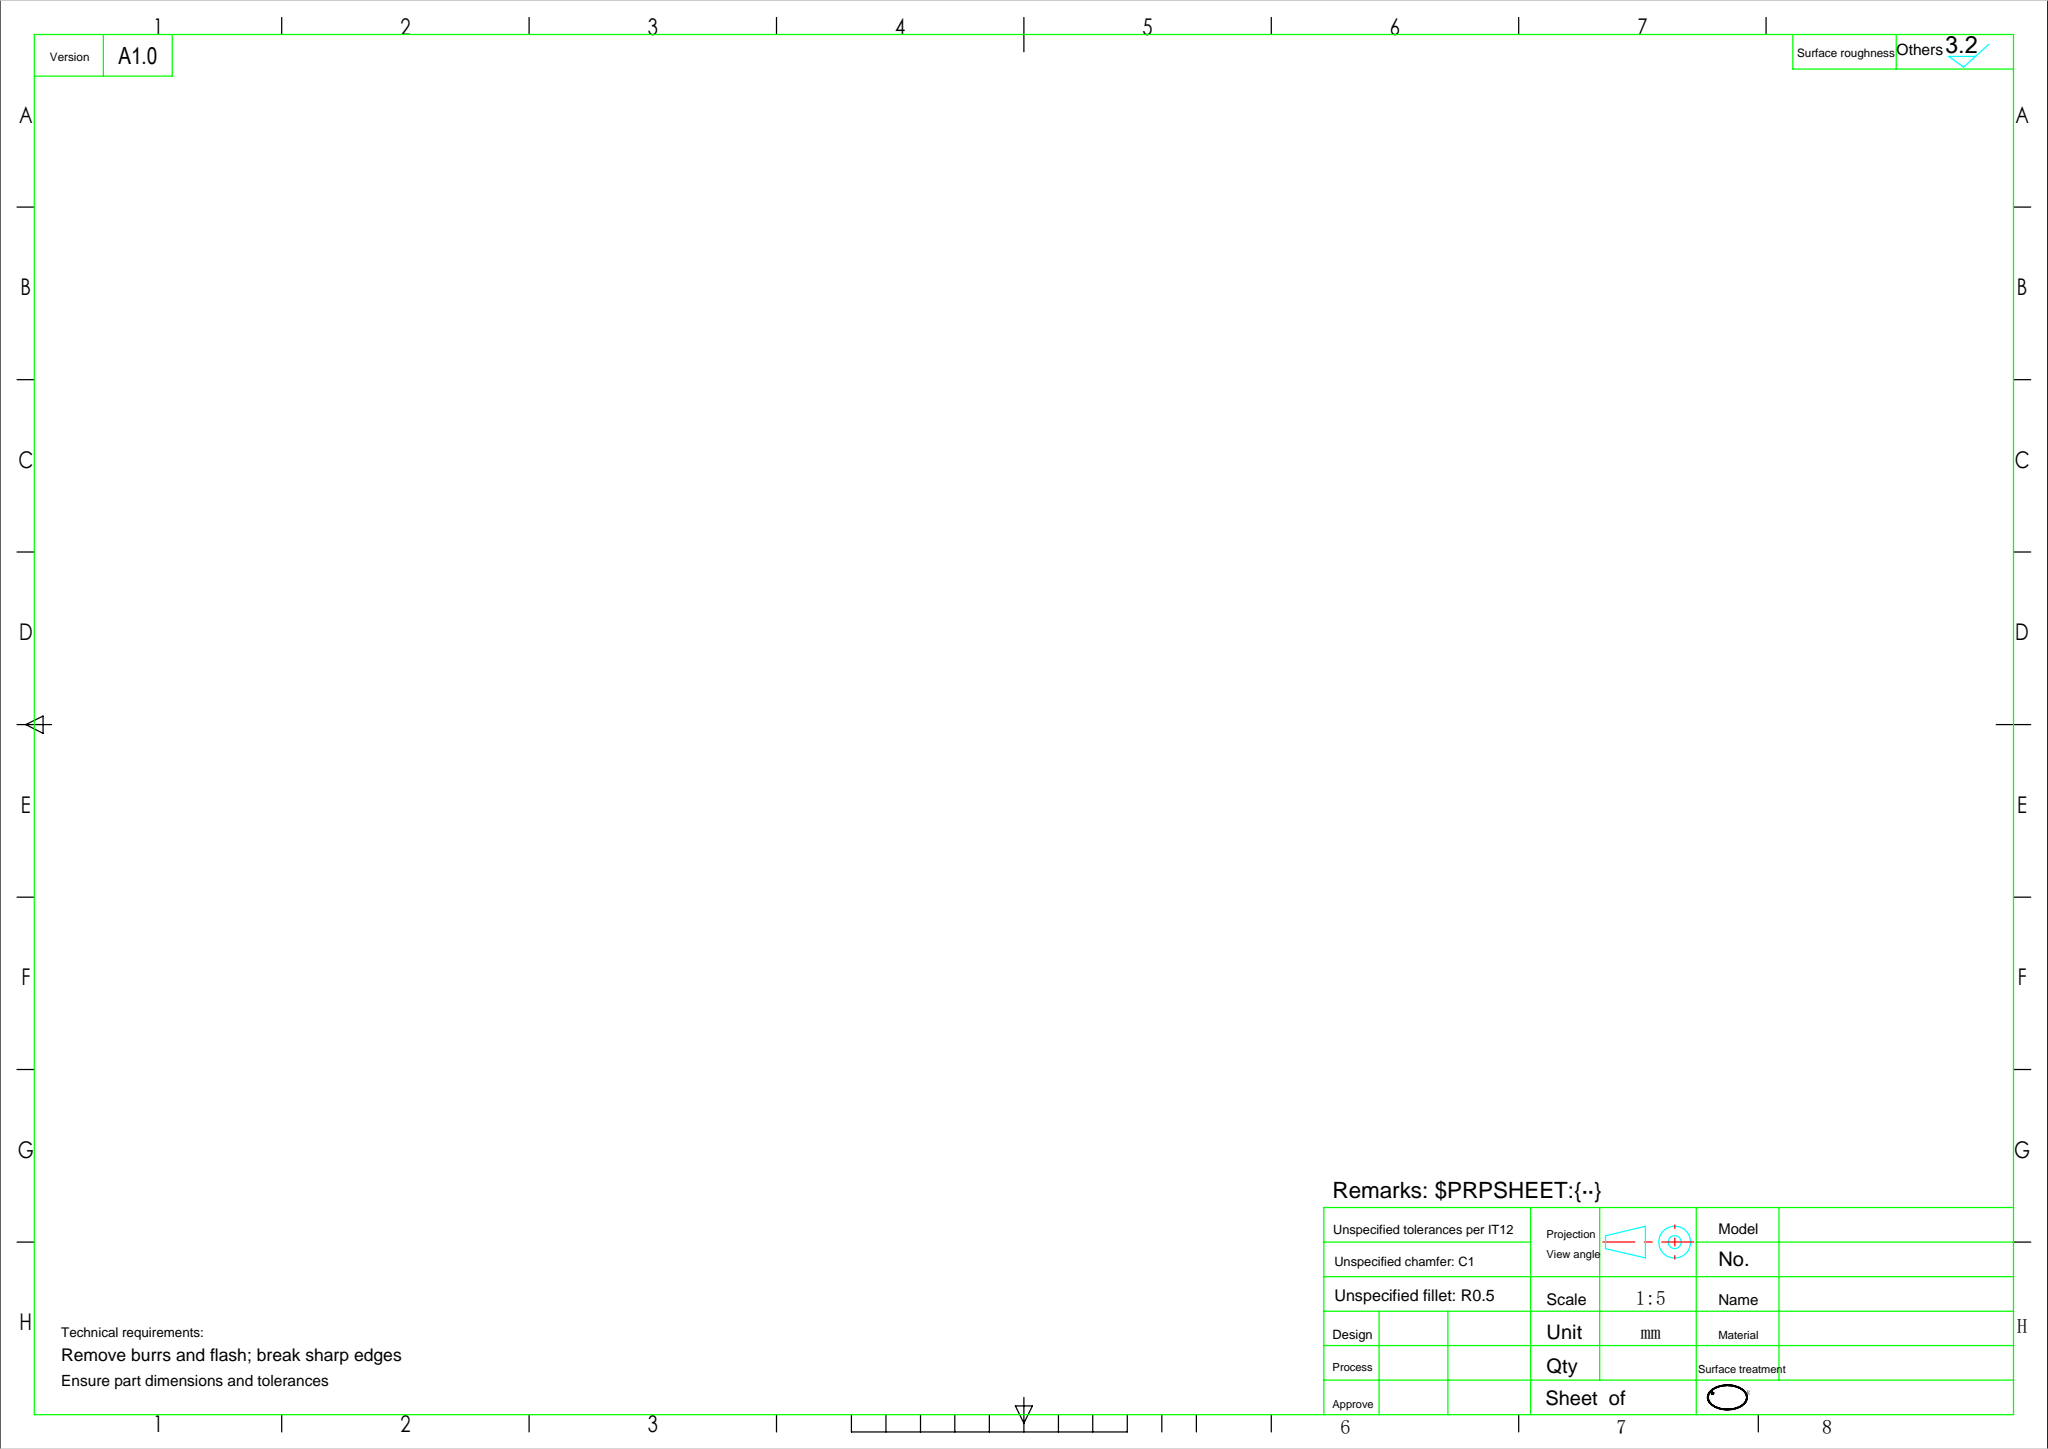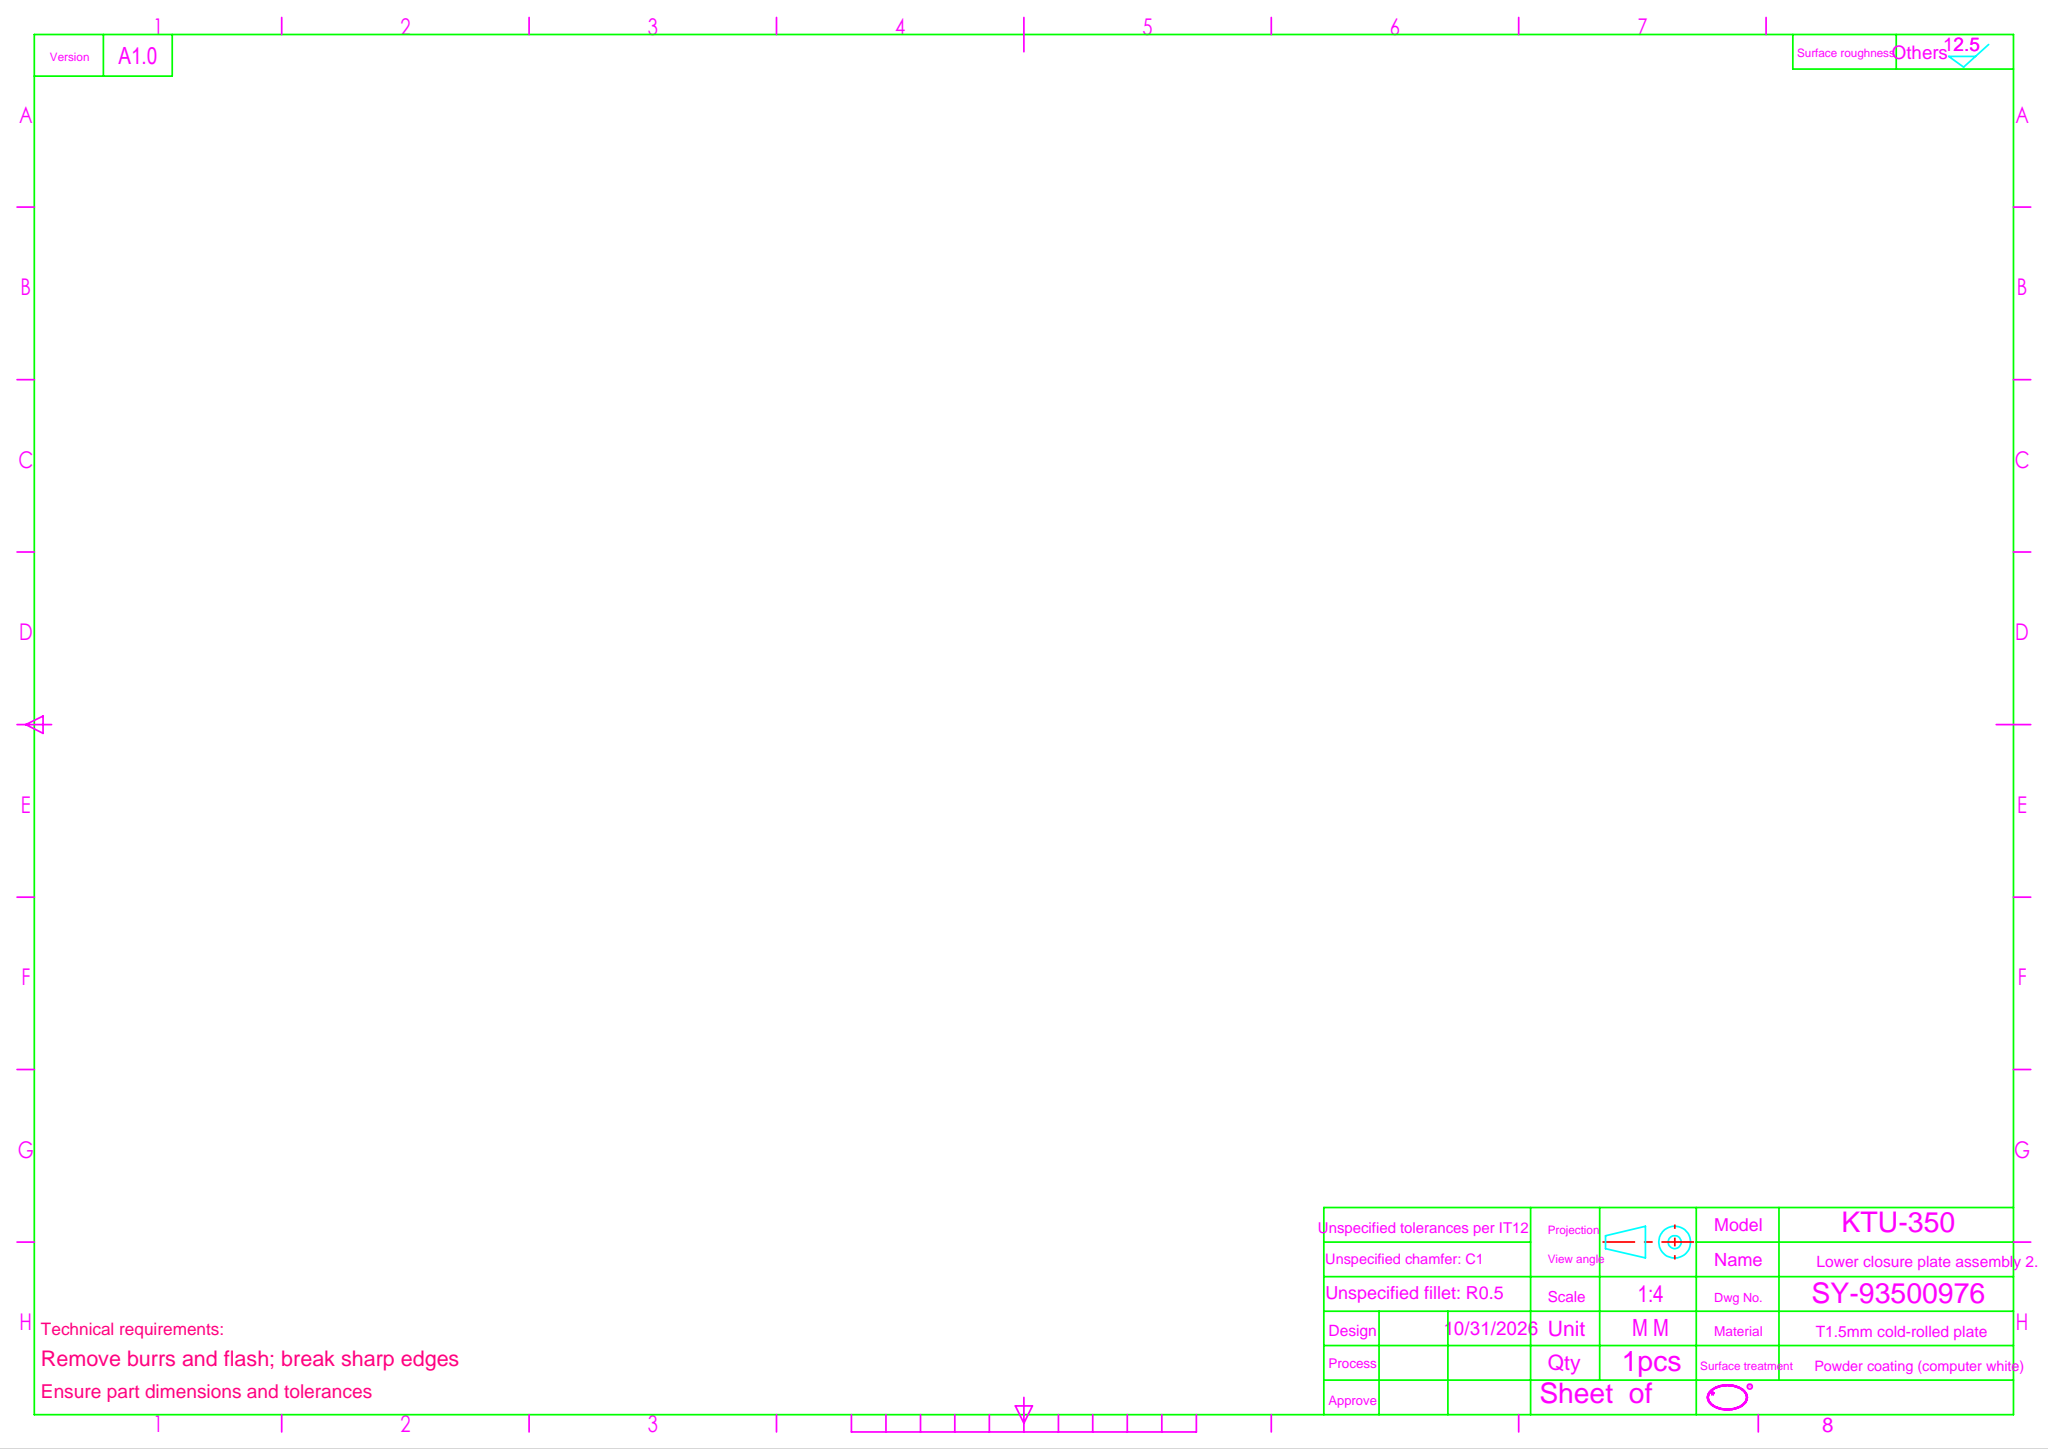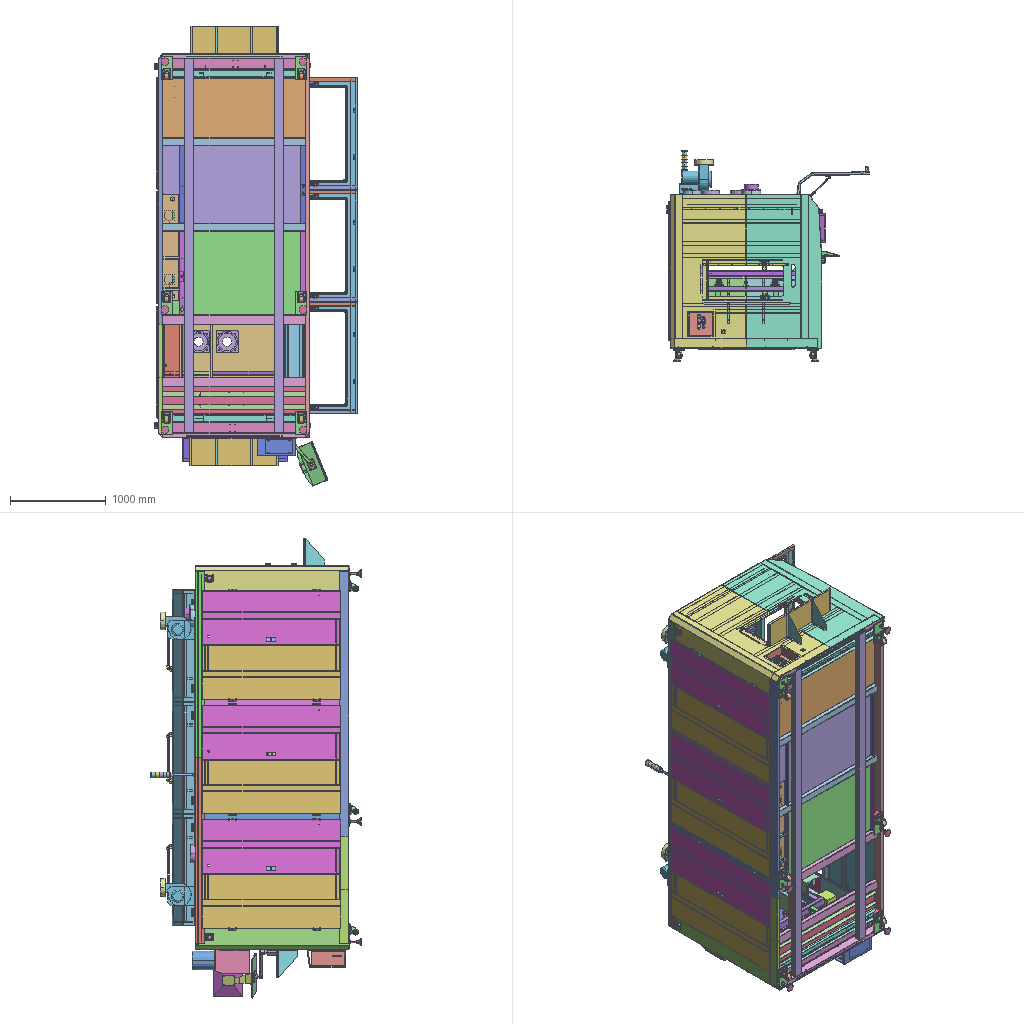Assembly | SolidWorks | 265 different items | 675 placed | box 2116 x 2194 x 4792 mm
Parts list (item | name | quantity | parent item | size | volume | features), first 143 of 265 items:
1 | (subassembly) | x1 | - | 221.2 x 220 x 250 mm | 34261 mm3 | -
2 | (subassembly) | x1 | in 42 | 110 x 260 x 135 mm | 170663 mm3 | features CompositeCurve 1
3 | (subassembly) | x6 | - | 70 x 60 x 101 mm | 39766 mm3 | -
4 | (subassembly) | x3 | in 35 | 1445 x 20 x 561.501 mm | 1629553 mm3 | -
5 | (subassembly) | x3 | in 29 | 57.054 x 67.632 x 37 mm | 10154 mm3 | -
6 | (subassembly) | x1 | in 39 | 430 x 207.698 x 23.832 mm | 300850 mm3 | -
7 | (subassembly) | x1 | in 32 | 170 x 309 x 179.5 mm | 344501 mm3 | -
8 | (subassembly) | x1 | in 32 | 165 x 165 x 31 mm | 59281 mm3 | -
9 | (subassembly) | x1 | in 39 | 106 x 70 x 75.939 mm | 90643 mm3 | -
10 | (subassembly) | x1 | in 39 | 120 x 64 x 180 mm | 129925 mm3 | -
11 | (subassembly) | x1 | in 18 | 1000 x 310 x 80 mm | 1097727 mm3 | -
12 | (subassembly) | x1 | in 39 | 40 x 74 x 370 mm | 161473 mm3 | -
13 | (subassembly) | x1 | - | 85 x 158 x 88 mm | 192242 mm3 | -
14 | (subassembly) | x6 | - | 82 x 93 x 113.3 mm | 232725 mm3 | -
15 | (subassembly) | x2 | - | 310.055 x 349.5 x 362 mm | 816455 mm3 | features CompositeCurve 1
16 | (subassembly) | x2 | - | 72.5 x 31.65 x 31.65 mm | 12632 mm3 | -
17 | (subassembly) | x1 | - | 1085 x 350 x 250 mm | 1083836 mm3 | -
18 | (subassembly) | x1 | in 20 | 1580 x 662 x 3996 mm | 37221159 mm3 | -
19 | (subassembly) | x1 | in 20 | 1580 x 269 x 1600 mm | 11681636 mm3 | -
20 | (subassembly) | x1 | - | - | 82035624 mm3 | features MirrorCompFeat 1, ReferencePattern 1
21 | (subassembly) | x1 | in 20 | 1580 x 269.314 x 1600 mm | 10508370 mm3 | features LocalLPattern 1
22 | (subassembly) | x1 | in 18 | 1000 x 550 x 80 mm | 1598201 mm3 | -
23 | (subassembly) | x1 | in 20 | 106 x 1320 x 3896 mm | 19791071 mm3 | features ReferencePattern 4, LocalLPattern 2
24 | (subassembly) | x3 | in 34 | 1445 x 21.5 x 592 mm | 1713091 mm3 | -
25 | (subassembly) | x1 | in 48 | 1110 x 1395 x 228 mm | 4724394 mm3 | features LayoutProfileFeature 1
26 | (subassembly) | x3 | - | 40.015 x 773.5 x 1165 mm | 1625267 mm3 | features InContextFeatHolder 2
27 | (subassembly) | x6 | - | 80 x 195 x 80 mm | 165012 mm3 | -
28 | (subassembly) | x2 | - | 60 x 70.5 x 60 mm | 57599 mm3 | -
29 | (subassembly) | x3 | - | 348.6 x 752.5 x 1165 mm | 4533101 mm3 | -
30 | (subassembly) | x1 | - | 900 x 20 x 2.5 mm | 44143 mm3 | -
31 | (subassembly) | x1 | - | 1000 x 35 x 2.5 mm | 51061 mm3 | -
32 | (subassembly) | x1 | - | 170 x 309 x 179.5 mm | 403796 mm3 | -
33 | (subassembly) | x2 | - | 69 x 71 x 68.718 mm | 90688 mm3 | -
34 | (subassembly) | x3 | - | 1445 x 21.5 x 610.75 mm | 1744268 mm3 | -
35 | (subassembly) | x3 | - | 1445 x 20.5 x 580.25 mm | 1660730 mm3 | -
36 | (subassembly) | x4 | - | 30.5 x 66.5 x 40 mm | 49373 mm3 | -
37 | (subassembly) | x2 | - | 59.341 x 58.854 x 51.237 mm | 55512 mm3 | -
38 | (subassembly) | x4 | - | 30.5 x 72 x 40 mm | 48162 mm3 | -
39 | (subassembly) | x1 | - | 300.234 x 578.209 x 672.62 mm | 4364638 mm3 | -
40 | (subassembly) | x10 | - | 86.5 x 28 x 16 mm | 25571 mm3 | -
41 | (subassembly) | x1 | - | 400.001 x 393 x 186.5 mm | 15923225 mm3 | -
42 | (subassembly) | x1 | - | 110 x 260 x 135 mm | 184897 mm3 | -
43 | (subassembly) | x3 | in 29 | 57.054 x 67.632 x 37 mm | 10154 mm3 | -
44 | (subassembly) | x2 | - | 251.752 x 77.5 x 127.178 mm | 270246 mm3 | -
45 | (subassembly) | x6 | - | 22 x 22 x 283.184 mm | 83831 mm3 | -
46 | (subassembly) | x12 | in 34, 35 | 47.323 x 29.106 x 79.396 mm | 15589 mm3 | -
47 | (subassembly) | x6 | in 29 | 62.892 x 24.747 x 79 mm | 32043 mm3 | -
48 | (subassembly) | x1 | - | 1110 x 1395 x 228 mm | 9072587 mm3 | features InContextFeatHolder 4, LayoutProfileFeature 1
49 | - | x4 | - | 290 x 208.5 x 20 mm | 66535 mm3 | features EdgeFlange 3, Fillet 3, ICE 3, FlatPattern 1, SMBaseFlange 1, SheetMetal 1
50 | - | x2 | in 20 | 180 x 145 x 5 mm | 69721 mm3 | features ICE 2, Fillet 1, FlatPattern 1, SMBaseFlange 1, SheetMetal 1
51 | - | x2 | in 20 | 210 x 140 x 5 mm | 73500 mm3 | features FlatPattern 1, SMBaseFlange 1, SheetMetal 1
52 | - | x1 | in 6 | 430 x 207.698 x 20.788 mm | 279577 mm3 | features EdgeFlange 5, Fillet 2, Chamfer 1, FlatPattern 1, HoleWzd 1, SMBaseFlange 1, SheetMetal 1
53 | - | x1 | in 6 | 75 x 12 x 110 mm | 20271 mm3 | features FlatPattern 1, HoleWzd 1, SMBaseFlange 1, SheetMetal 1
54 | - | x3 | in 19, 21 | 80 x 50 x 1498 mm | 1094858 mm3 | features ExtruThin 1
55 | - | x1 | in 21 | 80 x 50 x 1498 mm | 1081389 mm3 | features Cut 2, ICE 2, ExtruThin 1
56 | - | x1 | in 19 | 80 x 30 x 1200 mm | 269880 mm3 | features ICE 5, LPattern 2, Fillet 1, FlatPattern 1, HoleWzd 1, SMBaseFlange 1, SheetMetal 1
57 | - | x1 | in 21 | 80 x 30 x 1200 mm | 269880 mm3 | features MirrorStock 1
58 | - | x1 | in 19 | 80 x 30 x 1200 mm | 275646 mm3 | features ICE 3, HoleWzd 2, LPattern 2, Cut 1, Fillet 1, FlatPattern 1, SMBaseFlange 1, SheetMetal 1
59 | - | x1 | in 21 | 80 x 30 x 750 mm | 164546 mm3 | features ICE 5, HoleWzd 2, LPattern 2, Fillet 1, FlatPattern 1, SMBaseFlange 1, SheetMetal 1
60 | - | x3 | in 29 | 257 x 740 x 1165 mm | 1879483 mm3 | features Chamfer 10, ICE 7, FlatPattern 6, HoleWzd 5, SMBaseFlange 5, SheetMetal 5, Fillet 3, MirrorSolid 2, CornerFeat 1, EdgeFlange 1
61 | - | x1 | - | 350 x 320 x 2 mm | 222822 mm3 | features Fillet 1, FlatPattern 1, HoleWzd 1, ICE 1, LPattern 1, SMBaseFlange 1, SheetMetal 1
62 | - | x1 | - | 83 x 1200 x 8 mm | 134894 mm3 | features EdgeFlange 2, ICE 2, Fillet 1, FlatPattern 1, LPattern 1, SMBaseFlange 1, SheetMetal 1
63 | - | x2 | - | 78 x 20 x 1136 mm | 123990 mm3 | features ICE 2, Fillet 1, FlatPattern 1, LPattern 1, SMBaseFlange 1, SheetMetal 1
64 | - | x1 | - | 83 x 750 x 8 mm | 82624 mm3 | features ICE 2, EdgeFlange 1, Fillet 1, FlatPattern 1, LPattern 1, SMBaseFlange 1, SheetMetal 1
65 | - | x1 | in 7 | 159 x 246 x 159 mm | 241682 mm3 | features ICE 4, ExtruThin 1
66 | - | x1 | in 7 | 170 x 40 x 177 mm | 65584 mm3 | features EdgeFlange 1, Fillet 1, FlatPattern 1, ICE 1, LPattern 1, SMBaseFlange 1, SheetMetal 1
67 | - | x1 | in 7 | 170 x 45 x 90 mm | 25517 mm3 | features ICE 2, EdgeFlange 1, Fillet 1, FlatPattern 1, SMBaseFlange 1, SheetMetal 1
68 | - | x1 | in 8 | 165 x 165 x 10 mm | 25826 mm3 | features 3DProfileFeature 1, EdgeFlange 1, FlatPattern 1, ICE 1, SMBaseFlange 1, SheetMetal 1
69 | - | x1 | in 8 | 150 x 150 x 1.5 mm | 26025 mm3 | features CirPattern 2, ICE 2, FlatPattern 1, HoleWzd 1, SMBaseFlange 1, SheetMetal 1
70 | - | x1 | in 10 | 120 x 64 x 110 mm | 76419 mm3 | features FlatPattern 2, SMBaseFlange 2, SheetMetal 2, Fillet 1, ICE 1
71 | - | x3 | in 26 | 40.015 x 773.5 x 1165 mm | 1466617 mm3 | features EdgeFlange 3, Fillet 2, ICE 2, CornerFeat 1, FlatPattern 1, HoleWzd 1, SMBaseFlange 1, SheetMetal 1
72 | - | x1 | in 12 | 30 x 30 x 303.542 mm | 79870 mm3 | features ExtruThin 1, ICE 1
73 | - | x2 | in 12 | 40 x 40 x 2 mm | 2513 mm3 | features FlatPattern 1, SMBaseFlange 1, SheetMetal 1
74 | - | x1 | in 41 | 186.5 x 393 x 400.001 mm | 689190 mm3 | features ICE 5, EdgeFlange 3, LPattern 2, FlatPattern 1, SMBaseFlange 1, SheetMetal 1
75 | - | x4 | in 33, 44 | 52 x 16 x 52 mm | 16958 mm3 | features BaseBody 1
76 | - | x2 | in 15 | 50 x 190 x 190 mm | 56980 mm3 | features 3DProfileFeature 1, EdgeFlange 1, FlatPattern 1, SMBaseFlange 1, SheetMetal 1
77 | - | x2 | in 15 | 290.055 x 331.5 x 312 mm | 759476 mm3 | features ICE 9, Fillet 2, SMBaseFlange 2, SheetMetal 2, FlatPattern 1, Shell 1
78 | - | x2 | - | 100 x 88.5 x 20 mm | 10166 mm3 | features EdgeFlange 2, ICE 2, Fillet 1, FlatPattern 1, SMBaseFlange 1, SheetMetal 1
79 | - | x1 | in 13 | 49 x 48 x 26 mm | 15129 mm3 | features BaseBody 1
80 | - | x1 | in 13 | 38 x 7 x 38 mm | 3168 mm3 | features BaseBody 1
81 | - | x6 | in 14 | 55 x 63 x 63 mm | 157755 mm3 | features BaseBody 1
82 | - | x3 | in 29 | 5 x 448 x 985 mm | 2206390 mm3 | features Chamfer 1, ICE 1
83 | - | x6 | in 14 | 82 x 11 x 107 mm | 39892 mm3 | features BaseBody 1
84 | - | x6 | in 14 | 69 x 65.5 x 76.3 mm | 35082 mm3 | features BaseBody 1
85 | - | x6 | in 27 | 80 x 195 x 80 mm | 159151 mm3 | features BaseBody 1
86 | - | x6 | in 27 | 30 x 11 x 34.641 mm | 5861 mm3 | features BaseBody 1
87 | - | x1 | - | 290 x 290 x 106.5 mm | 187647 mm3 | features ICE 3, 3DProfileFeature 2, EdgeFlange 2, FlatPattern 2, SMBaseFlange 2, SheetMetal 2, Fillet 1
88 | - | x1 | in 30 | 900 x 20 x 1.5 mm | 26857 mm3 | features Fillet 1, FlatPattern 1, HoleWzd 1, ICE 1, LPattern 1, SMBaseFlange 1, SheetMetal 1
89 | - | x1 | in 30 | 870 x 20 x 1 mm | 17285 mm3 | features Fillet 1, FlatPattern 1, ICE 1, LPattern 1, SMBaseFlange 1, SheetMetal 1
90 | - | x1 | in 31 | 1000 x 35 x 1.5 mm | 31176 mm3 | features LPattern 2, SMBaseFlange 2, Fillet 1, FlatPattern 1, HoleWzd 1, ICE 1, SheetMetal 1
91 | - | x1 | in 31 | 1000 x 20 x 1 mm | 19885 mm3 | features Fillet 1, FlatPattern 1, ICE 1, LPattern 1, SMBaseFlange 1, SheetMetal 1
92 | - | x2 | in 16 | 13.5 x 13.5 x 1 mm | 61.426 mm3 | features FlatPattern 1, SMBaseFlange 1, SheetMetal 1
93 | - | x6 | in 29 | 986 x 22 x 8.2 mm | 33274 mm3 | features Chamfer 1, Fillet 1, FlatPattern 1, HoleWzd 1, SMBaseFlange 1, SheetMetal 1
94 | - | x2 | in 16 | 18.5 x 18.5 x 1 mm | 187.09 mm3 | features FlatPattern 1, SMBaseFlange 1, SheetMetal 1
95 | - | x2 | in 16 | 11.85 x 31.65 x 31.65 mm | 3001 mm3 | features ICE 2, Chamfer 1, Revolution 1
96 | - | x1 | - | 222 x 100 x 20 mm | 440921 mm3 | features Extrusion 1, ICE 1
97 | - | x12 | in 29 | 10 x 6.5 x 10 mm | 321.367 mm3 | features Chamfer 1, HoleWzd 1, Revolution 1
98 | - | x2 | in 19, 21 | 292 x 108 x 263 mm | 272152 mm3 | features ICE 9, MirrorPattern 3, EdgeFlange 2, 3DProfileFeature 1, Fillet 1, FlatPattern 1, HoleWzd 1, SMBaseFlange 1, SheetMetal 1
99 | - | x2 | - | 1470 x 70 x 28.335 mm | 610079 mm3 | features ICE 4, Extrusion 1
100 | - | x1 | - | 1.5 x 299 x 88 mm | 38958 mm3 | features ICE 2, SMBaseFlange 2, Fillet 1, FlatPattern 1, LPattern 1, SheetMetal 1
101 | - | x1 | - | 1.5 x 338 x 88 mm | 40889 mm3 | features ICE 2, Fillet 1, FlatPattern 1, SMBaseFlange 1, SheetMetal 1
102 | - | x4 | in 18 | 1480 x 100 x 50 mm | 1265578 mm3 | features HoleWzd 3, BaseBody 1, ICE 1, MoveFace 1
103 | - | x2 | in 18 | 1480 x 50 x 80 mm | 1087950 mm3 | features HoleWzd 2, BaseBody 1, ICE 1, MoveFace 1
104 | - | x2 | - | 227 x 1446 x 100 mm | 746223 mm3 | features EdgeFlange 4, HoleWzd 3, CornerFeat 1, Fillet 1, FlatPattern 1, SMBaseFlange 1, SheetMetal 1
105 | - | x2 | in 18 | 1480 x 48 x 100 mm | 1562650 mm3 | features BaseBody 1, Fillet 1, ICE 1, MoveFace 1
106 | - | x1 | in 19 | 30 x 93 x 303 mm | 47939 mm3 | features EdgeFlange 2, FlatPattern 1, HoleWzd 1, ICE 1, SMBaseFlange 1, SheetMetal 1
107 | - | x1 | in 21 | 35 x 343 x 93 mm | 61855 mm3 | features EdgeFlange 2, HoleWzd 2, ICE 2, FlatPattern 1, SMBaseFlange 1, SheetMetal 1
108 | - | x1 | in 17 | 1082 x 350 x 250 mm | 789625 mm3 | features HoleWzd 2, ICE 2, Fillet 1, FlatPattern 1, SMBaseFlange 1, SheetMetal 1
109 | - | x1 | in 17 | 40 x 350 x 250 mm | 147105 mm3 | features EdgeFlange 1, FlatPattern 1, ICE 1, SMBaseFlange 1, SheetMetal 1
110 | - | x1 | in 17 | 40 x 350 x 250 mm | 147105 mm3 | features EdgeFlange 1, FlatPattern 1, ICE 1, SMBaseFlange 1, SheetMetal 1
111 | - | x1 | - | 184.5 x 185 x 575 mm | 243873 mm3 | features ICE 4, Fillet 2, EdgeFlange 1, FlatPattern 1, LPattern 1, MoveFace 1, SMBaseFlange 1, SheetMetal 1
112 | - | x1 | - | 180 x 185 x 510 mm | 215412 mm3 | features Fillet 2, ICE 2, EdgeFlange 1, FlatPattern 1, LPattern 1, MoveFace 1, SMBaseFlange 1, SheetMetal 1
113 | - | x6 | in 4, 24 | 46 x 18 x 264 mm | 29896 mm3 | features Cut 1, FlatPattern 1, ICE 1, MirrorPattern 1, SMBaseFlange 1, SheetMetal 1
114 | - | x3 | in 25 | 1065 x 56 x 15 mm | 167971 mm3 | features EdgeFlange 2, ICE 2, Cut 1, Fillet 1, FlatPattern 1, HoleWzd 1, MoveFace 1, SMBaseFlange 1, SheetMetal 1
115 | - | x1 | - | 57 x 30 x 1815 mm | 185847 mm3 | features Fillet 1, FlatPattern 1, ICE 1, LPattern 1, SMBaseFlange 1, SheetMetal 1
116 | - | x1 | in 48 | 1097 x 1327 x 10 mm | 2209760 mm3 | features Cut 5, MoveFace 5, EdgeFlange 2, ICE 2, FlatPattern 1, HoleWzd 1, SMBaseFlange 1, SheetMetal 1
117 | - | x2 | - | 230 x 230 x 101.5 mm | 135571 mm3 | features BossThin 2, FlatPattern 1, ICE 1, SMBaseFlange 1, SheetMetal 1
118 | - | x2 | - | 250 x 250 x 100 mm | 145247 mm3 | features ICE 4, FlatPattern 1, SMBaseFlange 1, SheetMetal 1
119 | - | x1 | in 18 | 50 x 100 x 3996 mm | 4387971 mm3 | features HoleWzd 4, ICE 3, CombineBodies 2, Cut 2, ExtruThin 1, LPattern 1
120 | - | x2 | in 18 | 100 x 50 x 3896 mm | 4345591 mm3 | features ExtruThin 1
121 | - | x2 | in 18 | 106 x 1480 x 11.5 mm | 272266 mm3 | features Cut 2, FlatPattern 1, SMBaseFlange 1, SheetMetal 1
122 | - | x1 | in 19 | 263.5 x 789.9 x 1600 mm | 3203804 mm3 | features ICE 19, EdgeFlange 8, Cut 5, 3DProfileFeature 3, HoleWzd 3, FlatPattern 2, SMBaseFlange 2, SheetMetal 2
123 | - | x10 | in 19, 21 | 50 x 40 x 1230 mm | 329899 mm3 | features Cut 1, ExtruThin 1, HoleWzd 1
124 | - | x1 | in 21 | 233 x 789.9 x 1600 mm | 2696095 mm3 | features ICE 10, Cut 4, EdgeFlange 4, HoleWzd 4, 3DProfileFeature 2, FlatPattern 2, SMBaseFlange 2, SheetMetal 2, DelFace 1
125 | - | x1 | in 21 | 789.9 x 263.5 x 1600 mm | 2950026 mm3 | features ICE 17, EdgeFlange 8, Cut 5, FlatPattern 2, HoleWzd 2, SMBaseFlange 2, SheetMetal 2, 3DProfileFeature 1, DelFace 1
126 | - | x1 | in 22 | 1000 x 80 x 50 mm | 709790 mm3 | features Cut 2, ICE 2, Extrusion 1, Fillet 1, Shell 1
127 | - | x1 | in 23 | 100 x 50 x 3896 mm | 3291789 mm3 | features LPattern 6, HoleWzd 4, 3DProfileFeature 1, DelFace 1, ExtruThin 1
128 | - | x1 | in 23 | 60 x 30 x 3896 mm | 1913419 mm3 | features ExtruThin 1
129 | - | x1 | in 23 | 1947 x 300 x 106 mm | 1794702 mm3 | features Cut 7, EdgeFlange 5, HoleWzd 4, ICE 4, LPattern 2, 3DProfileFeature 1, FlatPattern 1, MirrorPattern 1, SMBaseFlange 1, SheetMetal 1
130 | - | x2 | in 23 | 30 x 30 x 3896 mm | 1212139 mm3 | features ExtruThin 1
131 | - | x1 | in 23 | 969 x 16 x 1947 mm | 3772126 mm3 | features ICE 5, Cut 3, EdgeFlange 1, FlatPattern 1, HoleWzd 1, MirrorPattern 1, SMBaseFlange 1, SheetMetal 1
132 | - | x1 | in 23 | 1947 x 300 x 100 mm | 1854038 mm3 | features Cut 8, EdgeFlange 5, HoleWzd 3, ICE 3, 3DProfileFeature 1, CirPattern 1, FlatPattern 1, LPattern 1, MirrorPattern 1, SMBaseFlange 1, SheetMetal 1
133 | - | x1 | in 23 | 969 x 16 x 1947 mm | 3707899 mm3 | features Cut 5, ICE 4, EdgeFlange 1, FlatPattern 1, MirrorPattern 1, SMBaseFlange 1, SheetMetal 1
134 | - | x2 | in 18 | 50 x 50 x 870 mm | 326788 mm3 | features Cut 1, FlatPattern 1, HoleWzd 1, SMBaseFlange 1, SheetMetal 1
135 | - | x2 | - | 25 x 90 x 20 mm | 7348 mm3 | features BaseBody 1, HoleWzd 1
136 | - | x3 | in 24 | 1445 x 21.5 x 592 mm | 1421822 mm3 | features EdgeFlange 3, Fillet 1, FlatPattern 1, HoleWzd 1, ICE 1, SMBaseFlange 1, SheetMetal 1
137 | - | x6 | in 20 | 110 x 40 x 40 mm | 58828 mm3 | features 3DProfileFeature 1, WeldMemberFeat 1, WeldmentFeature 1
138 | - | x3 | in 4 | 1445 x 20 x 561.501 mm | 1368180 mm3 | features ICE 4, EdgeFlange 2, FlatPattern 1, HoleWzd 1, SMBaseFlange 1, SheetMetal 1
139 | - | x3 | in 24 | 46 x 18 x 264 mm | 29896 mm3 | features Cut 1, FlatPattern 1, ICE 1, MirrorPattern 1, SMBaseFlange 1, SheetMetal 1
140 | - | x2 | in 18 | 50 x 50 x 814 mm | 309344 mm3 | features FlatPattern 1, HoleWzd 1, SMBaseFlange 1, SheetMetal 1
141 | - | x2 | in 18 | 50 x 50 x 1480 mm | 562525 mm3 | features Cut 2, FlatPattern 1, SMBaseFlange 1, SheetMetal 1
142 | - | x1 | in 25 | 1110 x 1395 x 213 mm | 3750548 mm3 | features ICE 11, Cut 4, CornerFeat 1, EdgeFlange 1, FlatPattern 1, MirrorPattern 1, MoveFace 1, SMBaseFlange 1, SheetMetal 1
143 | - | x1 | - | 680 x 1530 x 1 mm | 1035471 mm3 | features Cut 3, Fillet 1, FlatPattern 1, ICE 1, SMBaseFlange 1, SheetMetal 1
Mates (type | each side: item.copy, entity, surface, feature), first 295 of 900 lines:
In the top assembly
Coincident | 119.1 face plane Extrude-薄壁1 | 71.1 face plane Base-Flange 1 | 2 times
DistanceDim | 71.1 face plane Edge-Flange 1 | 122.1 face plane Edge-Flange 1
Coincident | 119.1 face plane Extrude-薄壁1 | 71.2 face plane Base-Flange 1 | 2 times
Coincident | 119.1 face plane Extrude-薄壁1 | 71.3 face plane Base-Flange 1 | 2 times
DistanceDim | 71.3 face plane Edge-Flange 1 | 125.1 face plane Edge-Flange 5
DistanceDim | 71.1 face plane Edge-Flange 1 | 71.2 face plane Edge-Flange 1
DistanceDim | 104.1 face plane Edge-Flange 4 | 119.1 face plane Extrude-薄壁1
Width | 104.1 face plane Edge-Flange 1 | 104.1 face plane Edge-Flange 1 | 71.1 face plane Edge-Flange 1 | 71.2 face plane Edge-Flange 1
DistanceDim | 104.2 face plane Edge-Flange 4 | 119.1 face plane Extrude-薄壁1
Width | 104.2 face plane Edge-Flange 1 | 104.2 face plane Edge-Flange 1 | 71.3 face plane Edge-Flange 1 | 71.2 face plane Edge-Flange 1
Coincident | 104.1 face plane Edge-Flange 1 | 220.1 face plane Base-Flange 1
Slot | 220.1 face cylinder Cut-Extrude 1 | 104.1 face cylinder M5 Tapped Hole 1
Parallel | 220.1 face plane Base-Flange 1 | 104.1 face plane Base-Flange 2
Coincident | 104.1 face plane Edge-Flange 1 | 220.2 face plane Base-Flange 1
Coincident | 220.1 face plane Base-Flange 1 | 220.2 face plane Base-Flange 1 | 2 times
Coincident | 104.2 face plane Edge-Flange 1 | 220.3 face plane Base-Flange 1
Coincident | 220.1 face plane Base-Flange 1 | 220.3 face plane Base-Flange 1
Coincident | 104.2 face plane Edge-Flange 1 | 220.4 face plane Base-Flange 1
Coincident | 220.3 face plane Base-Flange 1 | 220.4 face plane Base-Flange 1 | 2 times
Coincident | 220.1 face plane Base-Flange 1 | 220.5 face plane Base-Flange 1 | 2 times
Concentric | 209.1 face cylinder Cut-Extrude 3 | 212.1 face cylinder Boss-Extrude 1
Coincident | 209.1 face plane Cut-Extrude 3 | 212.1 face plane Boss-Extrude 1
Concentric | 179.1 face cylinder Cut-Extrude 2 | 209.1 face cylinder Cut-Extrude 1
Coincident | 179.1 face plane Cut-Extrude 1 | 209.1 face plane Cut-Extrude 1
Concentric | 212.2 face cylinder Boss-Extrude 1 | 209.2 face cylinder Cut-Extrude 3
Coincident | 212.2 face plane Boss-Extrude 1 | 209.2 face plane Cut-Extrude 3
Concentric | 179.2 face cylinder Cut-Extrude 2 | 209.2 face cylinder Cut-Extrude 1
Coincident | 247.1 face plane Extrude-薄壁1 | 142.1 face plane Edge-Flange 1
DistanceDim | 253.1 face plane Extrude-薄壁1 | 142.1 face plane Base-Flange 1
DistanceDim | 142.1 face plane Edge-Flange 1 | 249.1 face plane Base-Flange 1
Coincident | 129.1 face plane Edge-Flange 2 | 194.1 face plane 输入1
DistanceDim | 194.1 face plane 输入1 | 129.1 face plane Edge-Flange 1
Coincident | 247.1 face plane Extrude-薄壁1 | 194.2 face plane 输入1
DistanceDim | 194.2 face plane 输入1 | 247.1 face plane Extrude-薄壁1
Coincident | 247.1 face plane Extrude-薄壁1 | 194.3 face plane 输入1
Coincident | 194.2 face plane 输入1 | 194.3 face plane 输入1
Coincident | 125.1 face plane Base-Flange 1 | 108.1 face plane Base-Flange 1
DistanceDim | 108.1 face plane Base-Flange 1 | 125.1 face plane Cut-Extrude 4
DistanceDim | 109.1 face plane Base-Flange 1 | 125.1 face plane Cut-Extrude 4
Coincident | 131.1 face plane Base-Flange 1 | 77.1 face plane Base-Flange 1
Coincident | 107.1 face plane Base-Flange 1 | 101.1 face plane Base-Flange 1
Coincident | 54.1 face plane Extrude-薄壁1 | 232.1 face plane Base-Flange 1
Slot | 227.1 face plane Cut-Extrude 1 | 228.1 face cylinder M4 Tapped Hole 1
Slot | 228.1 face cylinder M4 Tapped Hole 1 | 227.1 face plane Cut-Extrude 1
Coincident | 227.1 face plane Base-Flange 1 | 228.1 face plane Base-Flange 1
Coincident | 227.1 face plane Base-Flange 1 | 228.2 face plane Base-Flange 1
Slot | 228.2 face cylinder M4 Tapped Hole 1 | 227.1 face plane Cut-Extrude 1 | 2 times
Slot | 228.1 face plane Cut-Extrude 1 | 98.1 face cylinder Cut-Extrude 3 | 2 times
Coincident | 98.1 face plane Base-Flange 1 | 228.1 face plane Base-Flange 1
Coincident | 240.1 face plane Base-Flange 1 | 238.1 face plane Edge-Flange 1
Concentric | 238.1 face cylinder M4 Tapped Hole 1 | 240.1 face cylinder Cut-Extrude 3 | 2 times
DistanceDim | 77.1 face plane Boss-Extrude 3 | 130.1 face plane Extrude-薄壁1
Slot | 127.1 face cylinder M6 Tapped Hole 2 | 254.1 face plane Cut-Extrude 3
Slot | 254.1 face plane Cut-Extrude 3 | 127.1 face cylinder M6 Tapped Hole 2 | 2 times
Coincident | 103.1 face plane 输入1 | 143.1 face plane Base-Flange 1
Coincident | 102.1 face plane 输入1 | 146.1 face plane Base-Flange 1
Coincident | 102.2 face plane 输入1 | 145.1 face plane Base-Flange 1
Parallel | 103.2 face plane 输入1 | 144.1 face plane Base-Flange 1
Coincident | 144.1 face plane Base-Flange 1 | 145.1 face plane Base-Flange 1
Parallel | 119.1 face plane Extrude-薄壁1 | 145.1 face plane Base-Flange 1
DistanceDim | 145.1 face plane Base-Flange 1 | 119.1 face plane Extrude-薄壁1
Coincident | 132.1 face plane Base-Flange 2 | 77.2 face plane Base-Flange 1
Coincident | 77.1 face plane Boss-Extrude 2 | 77.2 face plane Boss-Extrude 2
Coincident | 131.1 face plane Base-Flange 1 | 118.1 face plane Base-Flange 1
Concentric | 131.1 face cylinder Boss-Extrude 1 | 118.1 face cylinder Cut-Extrude 1 | 2 times
Coincident | 124.1 face plane Base-Flange 1 | 239.1 face plane Edge-Flange 2
Concentric | 124.1 face cylinder Cut-Extrude 8 | 173.1 face cylinder Boss-Extrude 1
Coincident | 124.1 face plane Base-Flange 1 | 173.1 face plane Boss-Extrude 2
Concentric | 124.1 face cylinder Cut-Extrude 8 | 239.1 face cylinder Cut-Extrude 1 | 2 times
Coincident | 149.1 face plane Base-Flange 1 | 239.2 face plane Edge-Flange 2
Concentric | 149.1 face cylinder Cut-Extrude 7 | 239.2 face cylinder Cut-Extrude 1 | 2 times
Coincident | 149.1 face plane Base-Flange 1 | 173.2 face plane Boss-Extrude 2
Concentric | 149.1 face cylinder Cut-Extrude 7 | 173.2 face cylinder Boss-Extrude 2
Coincident | 149.1 face plane Base-Flange 1 | 246.1 face plane Base-Flange 1
Concentric | 149.1 face cylinder Cut-Extrude 8 | 246.1 face cylinder Base-Flange 1 | 2 times
Coincident | 122.1 face plane Edge-Flange 4 | 135.1 face plane 输入1
Concentric | 122.1 face cylinder M5 Tapped Hole 1 | 135.1 face cylinder 输入1
Parallel | 122.1 face plane Edge-Flange 4 | 135.1 face plane 输入1
Coincident | 125.1 face plane Edge-Flange 8 | 135.2 face plane 输入1
Concentric | 125.1 face cylinder Cut-Extrude 12 | 135.2 face cylinder 输入1
Parallel | 125.1 face plane Edge-Flange 8 | 135.2 face plane 输入1
Coincident | 123.1 face plane Extrude-薄壁1 | 61.1 face plane Base-Flange 1
DistanceDim | 54.1 face plane Extrude-薄壁1 | 61.1 face plane Base-Flange 1
Coincident | 222.1 face plane Edge-Flange 1 | 61.1 face plane Base-Flange 1
Concentric | 222.1 face cylinder Ø6.0 (6) DiameterHole 1 | 61.1 face cylinder M5 Tapped Hole 1 | 2 times
DistanceDim | 150.1 face plane Base-Flange 1 | 229.1 face plane Base-Flange 1
Concentric | 150.1 face cylinder M5 Tapped Hole 1 | 229.1 face cylinder Cut-Extrude 1
Parallel | 150.1 face plane Base-Flange 1 | 229.1 face plane Base-Flange 1
Coincident | 150.2 face plane Base-Flange 1 | 229.2 face plane Base-Flange 1
Concentric | 150.2 face cylinder M5 Tapped Hole 1 | 229.2 face cylinder Cut-Extrude 1
Parallel | 150.2 face plane Base-Flange 1 | 229.2 face plane Base-Flange 1
Coincident | 56.1 face plane Base-Flange 1 | 151.1 face plane Base-Flange 1
Slot | 151.1 face cylinder Cut-Extrude 1 | 56.1 face cylinder M4 Tapped Hole 1
Parallel | 56.1 face plane Base-Flange 1 | 151.1 face plane Edge-Flange 1
Coincident | 58.1 face plane Base-Flange 1 | 62.1 face plane Base-Flange 1
Slot | 62.1 face cylinder Cut-Extrude 1 | 58.1 face cylinder M4 Tapped Hole 1
Parallel | 58.1 face plane Base-Flange 1 | 62.1 face plane Edge-Flange 2
Coincident | 150.2 face plane Base-Flange 1 | 63.1 face plane Base-Flange 1 | 2 times
Coincident | 150.1 face plane Base-Flange 1 | 63.2 face plane Base-Flange 1 | 2 times
Coincident | 59.1 face plane Base-Flange 1 | 64.1 face plane Base-Flange 1
Slot | 64.1 face cylinder Cut-Extrude 1 | 59.1 face cylinder M4 Tapped Hole 1
Parallel | 59.1 face plane Base-Flange 1 | 64.1 face plane Edge-Flange 1
Coincident | 57.1 face plane | 151.2 face plane Base-Flange 1
Slot | 151.2 face cylinder Cut-Extrude 1 | 57.1 face cylinder
Parallel | 57.1 face plane | 151.2 face plane Edge-Flange 1
Coincident | 129.1 face plane Edge-Flange 3 | 152.1 face plane Base-Flange 1
Coincident | 129.1 face plane Cut-Extrude 8 | 152.1 face plane Base-Flange 1
Coincident | 129.1 face plane Edge-Flange 2 | 152.1 face plane Base-Flange 1
Coincident | 132.1 face plane Edge-Flange 3 | 115.1 face plane Base-Flange 1
Coincident | 132.1 face plane Edge-Flange 2 | 115.1 face plane Base-Flange 1
Coincident | 132.1 face plane Cut-Extrude 10 | 115.1 face plane Base-Flange 1
Coincident | 58.1 face plane Base-Flange 1 | 112.1 face plane Base-Flange 1
Slot | 112.1 face cylinder Cut-Extrude 1 | 58.1 face cylinder M4 Tapped Hole 2
Parallel | 112.1 face plane Base-Flange 1 | 62.1 face plane Base-Flange 1
Coincident | 59.1 face plane Base-Flange 1 | 111.1 face plane Base-Flange 1
Slot | 111.1 face cylinder Cut-Extrude 1 | 59.1 face cylinder M4 Tapped Hole 2
Parallel | 111.1 face plane Base-Flange 1 | 64.1 face plane Base-Flange 1
DistanceDim | 144.1 face plane Base-Flange 1 | 145.1 face plane Base-Flange 1
DistanceDim | 143.1 face plane Base-Flange 1 | 144.1 face plane Base-Flange 1
DistanceDim | 145.1 face plane Base-Flange 1 | 102.2 face plane 输入1
DistanceDim | 146.1 face plane Base-Flange 1 | 102.1 face plane 输入1
Coincident | 145.1 face plane Base-Flange 1 | 146.1 face plane Base-Flange 1
Coincident | 55.1 face plane Extrude-薄壁1 | 153.1 face plane Edge-Flange 3
Parallel | 55.1 face plane Extrude-薄壁1 | 153.1 face plane Base-Flange 1
Coincident | 124.1 face plane Base-Flange 1 | 188.1 face plane 输入1
Concentric | 124.1 face cylinder M4 Tapped Hole 1 | 188.1 face cylinder 输入1
Parallel | 124.1 face plane Base-Flange 1 | 188.1 face plane 输入1
Coincident | 249.1 face plane Base-Flange 1 | 188.2 face plane 输入1
Concentric | 249.1 face cylinder Cut-Extrude 1 | 188.2 face cylinder 输入1 | 2 times
Concentric | 107.1 face cylinder M4 Tapped Hole 1 | 101.1 face cylinder Cut-Extrude 2 | 2 times
Coincident | 220.5 face plane Base-Flange 1 | 135.1 face plane 输入1
Coincident | 102.2 face plane 输入1 | 99.1 face plane Boss-Extrude 1 | 2 times
DistanceDim | 99.1 face plane Boss-Extrude 1 | 247.1 face plane Extrude-薄壁1
Coincident | 102.1 face plane 输入1 | 99.2 face plane Boss-Extrude 1 | 2 times
Coincident | 99.1 face plane Boss-Extrude 1 | 99.2 face plane Boss-Extrude 1
Coincident | 149.1 face plane Base-Flange 1 | 172.1 face plane Boss-Extrude 1
Concentric | 173.2 face cylinder Boss-Extrude 2 | 172.1 face cylinder Cut-Extrude 3
Parallel | 149.1 face plane Base-Flange 1 | 172.1 face plane Boss-Extrude 1
DistanceDim | 179.2 face plane Cut-Extrude 1 | 209.2 face plane Cut-Extrude 1
DistanceDim | 127.1 face plane Extrude-薄壁1 | 254.1 face plane Base-Flange 1
Coincident | 131.1 face plane Base-Flange 1 | 87.1 face plane Base-Flange 1
Concentric | 118.1 face cylinder Boss-Extrude 1 | 87.1 face cylinder Edge-Flange 1
Concentric | 131.1 face cylinder Boss-Extrude 1 | 87.1 face cylinder Cut-Extrude 2
Coincident | 125.1 face plane Base-Flange 1 | 74.1 face plane Edge-Flange 1
Concentric | 125.1 face cylinder Cut-Extrude 18 | 74.1 face cylinder Cut-Extrude 3
Parallel | 125.1 face plane Base-Flange 1 | 74.1 face plane Edge-Flange 2
Coincident | 61.1 face plane Base-Flange 1 | 67.1 face plane Edge-Flange 1
Concentric | 61.1 face cylinder M5 Tapped Hole 1 | 67.1 face cylinder Cut-Extrude 1
Parallel | 61.1 face plane Base-Flange 1 | 67.1 face plane Base-Flange 1
Coincident | 122.1 face plane Base-Flange 1 | 88.1 face plane Base-Flange 1
DistanceDim | 88.1 face plane Base-Flange 1 | 122.1 face plane Cut-Extrude 4
Width | 149.1 face plane Cut-Extrude 4 | 122.1 face plane Cut-Extrude 4 | 88.1 face plane Base-Flange 1 | 88.1 face plane Base-Flange 1
Coincident | 226.1 face plane Base-Flange 1 | 90.1 face plane Base-Flange 1
DistanceDim | 226.1 face plane Base-Flange 1 | 90.1 face plane Base-Flange 1
Coincident | 244.1 face plane | 261.1 face plane Edge-Flange 3
Coincident | 177.1 edge | 261.1 face plane Base-Flange 1
Coincident | 244.1 face plane | 177.1 edge | 2 times
DistanceDim | 261.1 face plane Edge-Flange 4 | 149.1 face plane Base-Flange 1
Coincident | 177.1 edge | 261.1 edge
Coincident | 125.1 face plane Base-Flange 1 | 70.1 face plane Base-Flange 1
Concentric | 125.1 face cylinder Cut-Extrude 7 | 70.1 face cylinder Cut-Extrude 1
Parallel | 125.1 face plane Base-Flange 1 | 70.1 face plane Base-Flange 1
DistanceDim | 61.1 face plane Base-Flange 1 | 123.1 face plane Extrude-薄壁1
Width | 125.1 face plane Cut-Extrude 4 | 124.1 face plane Cut-Extrude 2 | 90.1 face plane Base-Flange 1 | 90.1 face plane Base-Flange 1
Coincident | 106.1 face plane Base-Flange 1 | 100.1 face plane Base-Flange 1
Concentric | 106.1 face cylinder M4 Tapped Hole 1 | 100.1 face cylinder Cut-Extrude 2 | 2 times
Coincident | 108.1 face plane Base-Flange 1 | 217.1 face plane 曲Face-输入4
Concentric | 218.1 face cylinder 输入1 | 108.1 edge
Parallel | 125.1 face plane Base-Flange 1 | 217.1 face plane 曲Face-输入4
Parallel | 179.3 face plane Cut-Extrude 1 | 179.4 face plane Cut-Extrude 1
Slot | 194.1 face cylinder 输入1 | 129.1 face cylinder M4 Tapped Hole 2
DistanceDim | 194.2 face plane 输入1 | 194.3 face plane 输入1
Coincident | 143.1 face plane Base-Flange 1 | 144.1 face plane Base-Flange 1
Coincident | 124.1 face plane Base-Flange 1 | 172.2 face plane Boss-Extrude 1
Concentric | 173.1 face cylinder Boss-Extrude 2 | 172.2 face cylinder Cut-Extrude 3
Concentric | 125.1 face cylinder Cut-Extrude 24 | 183.1 face cylinder Imported1
Coincident | 125.1 face plane Base-Flange 2 | 181.1 face plane Imported1
Concentric | 122.1 face cylinder Cut-Extrude 13 | 183.2 face cylinder Imported1
Coincident | 122.1 face plane Base-Flange 2 | 181.2 face plane Imported1
Concentric | 101.1 face cylinder Cut-Extrude 1 | 166.1 face cylinder Imported1
Coincident | 101.1 face plane Base-Flange 1 | 166.1 face plane Imported1
Coincident | 101.1 face plane Base-Flange 1 | 175.1 face plane Imported1
Concentric | 101.1 face cylinder Cut-Extrude 1 | 175.1 face cylinder Imported1
Coincident | 101.1 face plane Base-Flange 1 | 167.1 face plane Imported1
Concentric | 101.1 face cylinder Cut-Extrude 1 | 167.1 face cylinder Imported1
Coincident | 100.1 face plane Base-Flange 1 | 167.2 face plane Imported1
Concentric | 100.1 face cylinder Cut-Extrude 1 | 167.2 face cylinder Imported1
Coincident | 132.1 face plane Base-Flange 2 | 157.1 face plane Boss-Extrude 10
Concentric | 132.1 face cylinder Cut-Extrude 4 | 157.1 face cylinder Boss-Extrude 9
DistanceDim | 127.1 face plane Extrude-薄壁1 | 104.1 face plane Edge-Flange 2
Coincident | 104.1 face plane Base-Flange 2 | 104.2 face plane Base-Flange 2
Coincident | 136.1 face plane Base-Flange 1 | 136.2 face plane Base-Flange 1
Concentric | 249.1 face cylinder Cut-Extrude 1 | 188.3 face cylinder 输入1 | 2 times
Coincident | 136.3 face plane Base-Flange 1 | 138.1 face plane Base-Flange 1
Concentric | 250.1 face cylinder | 188.4 face cylinder 输入1 | 2 times
Width | 195.1 face plane 输入1 | 195.2 face plane 输入1 | 113.1 face plane Base-Flange 1 | 113.2 face plane Base-Flange 1
Coincident | 220.1 face plane Base-Flange 1 | 220.4 face plane Base-Flange 1
Coincident | 220.6 face plane Base-Flange 1 | 135.2 face plane 输入1
Coincident | 220.5 face plane Base-Flange 1 | 220.6 face plane Base-Flange 1 | 2 times
DistanceDim | 150.2 face plane Base-Flange 1 | 63.1 face plane Base-Flange 1
DistanceDim | 150.1 face plane Base-Flange 1 | 63.2 face plane Base-Flange 1
DistanceDim | 258.1 face plane Base-Flange 1 | 77.1 face plane Base-Flange 1
Coincident | 55.1 face plane Extrude-薄壁1 | 153.1 face plane Base-Flange 1
Coincident | 122.1 face plane Base-Flange 1 | 78.1 face plane Base-Flange 1
Parallel | 122.1 face plane Cut-Extrude 4 | 78.1 face plane Edge-Flange 1
Coincident | 122.1 face plane Base-Flange 1 | 78.2 face plane Base-Flange 1
Parallel | 122.1 face plane Cut-Extrude 4 | 78.2 face plane Edge-Flange 1
Coincident | 126.1 face plane Boss-Extrude 1 | 159.1 face plane Boss-Extrude 1
Parallel | 126.1 face plane Boss-Extrude 1 | 159.1 face plane Boss-Extrude 1
Coincident | 126.1 face plane Boss-Extrude 1 | 159.2 face plane Boss-Extrude 1
Parallel | 126.1 face plane Boss-Extrude 1 | 159.2 face plane Boss-Extrude 1
Coincident | 197.1 face plane Boss-Extrude 1 | 159.3 face plane Boss-Extrude 1
Parallel | 197.1 face plane Boss-Extrude 1 | 159.3 face plane Boss-Extrude 1
Coincident | 197.1 face plane Boss-Extrude 1 | 159.4 face plane Boss-Extrude 1
Parallel | 197.1 face plane Boss-Extrude 1 | 159.4 face plane Boss-Extrude 1
Coincident | 197.1 face plane Boss-Extrude 1 | 241.1 face plane Boss-Extrude 1
Parallel | 197.1 face plane Boss-Extrude 1 | 241.1 face plane Boss-Extrude 1
Coincident | 126.1 face plane Boss-Extrude 1 | 241.2 face plane Boss-Extrude 1
Parallel | 126.1 face plane Boss-Extrude 1 | 241.2 face plane Boss-Extrude 1
Concentric | 241.2 face cylinder Cut-Extrude 3 | 154.1 face cylinder Boss-Extrude 3
Concentric | 241.1 face cylinder Cut-Extrude 3 | 154.2 face cylinder Boss-Extrude 3
Slot | 241.2 face cylinder Cut-Extrude 1 | 126.1 face cylinder Cut-Extrude 4 | 2 times
Coincident | 122.1 face plane Base-Flange 1 | 49.1 face plane Edge-Flange 1
Coincident | 149.1 face plane Base-Flange 1 | 49.2 face plane Edge-Flange 1
Coincident | 49.1 face plane Edge-Flange 2 | 49.2 face plane Edge-Flange 2
Coincident | 124.1 face plane Base-Flange 1 | 49.3 face plane Edge-Flange 1
Coincident | 125.1 face plane Base-Flange 1 | 49.4 face plane Edge-Flange 1
Coincident | 49.3 face plane Edge-Flange 2 | 49.4 face plane Edge-Flange 2
Coincident | 49.3 face plane Edge-Flange 2 | 242.1 face plane Base-Flange 1
Coincident | 49.3 face plane Edge-Flange 14 | 242.1 face plane Edge-Flange 1
Coincident | 49.1 face plane Edge-Flange 2 | 242.2 face plane Base-Flange 1
Coincident | 49.1 face plane Edge-Flange 14 | 242.2 face plane Edge-Flange 1
Slot | 49.3 face cylinder Cut-Extrude 4 | 124.1 face cylinder Cut-Extrude 14
Slot | 49.4 face cylinder Cut-Extrude 4 | 125.1 face cylinder Cut-Extrude 26
Slot | 49.2 face cylinder Cut-Extrude 4 | 149.1 face cylinder Cut-Extrude 12
Slot | 49.1 face cylinder Cut-Extrude 4 | 122.1 face cylinder Cut-Extrude 16
Slot | 78.1 face cylinder Cut-Extrude 2 | 122.1 face cylinder Cut-Extrude 15 | 2 times
Slot | 78.2 face cylinder Cut-Extrude 2 | 122.1 face cylinder Cut-Extrude 15 | 2 times
Coincident | 247.1 face plane 分割线1 | 194.4 face plane 输入1
DistanceDim | 195.3 face plane 输入1 | 247.1 face plane 分割线1
Coincident | 241.2 face plane Boss-Extrude 1 | 155.1 face plane Boss-Extrude 1
Coincident | 122.1 face plane Base-Flange 2 | 96.1 face plane Boss-Extrude 1
Concentric | 122.1 face cylinder Cut-Extrude 22 | 96.1 face cylinder Cut-Extrude 1 | 2 times
Concentric | 133.1 face cylinder Cut-Extrude 2 | 117.1 face cylinder Extrude-薄壁1
Coincident | 133.1 face plane Base-Flange 1 | 117.1 face plane Base-Flange 1
Concentric | 197.1 face cylinder Cut-Extrude 1 | 159.4 face cylinder Cut-Extrude 1
Concentric | 197.1 face cylinder Cut-Extrude 2 | 159.4 face cylinder Cut-Extrude 2
Slot | 241.1 face cylinder Cut-Extrude 1 | 197.1 face cylinder Cut-Extrude 3 | 2 times
Coincident | 241.1 face plane Boss-Extrude 1 | 155.2 face plane Boss-Extrude 1
Concentric | 126.1 face cylinder Cut-Extrude 2 | 159.2 face cylinder Cut-Extrude 1
Concentric | 126.1 face cylinder Cut-Extrude 2 | 159.1 face cylinder Cut-Extrude 1
Concentric | 197.1 face cylinder Cut-Extrude 1 | 159.3 face cylinder Cut-Extrude 1
Concentric | 197.1 face cylinder Cut-Extrude 2 | 159.4 face cylinder Cut-Extrude 3
Coincident | 98.2 face plane Base-Flange 1 | 79.1 face plane 输入1
Slot | 79.1 face cylinder 输入1 | 98.2 face cylinder M6 Tapped Hole 1 | 2 times
Concentric | 207.1 face cylinder Boss-Extrude 1 | 85.1 face cylinder 输入1
Coincident | 207.1 face plane Boss-Extrude 1 | 86.1 face plane 输入1
Coincident | 207.1 face plane Boss-Extrude 1 | 83.1 face plane 输入1
Slot | 83.1 face cylinder 输入1 | 207.1 face cylinder Boss-Extrude 1 | 2 times
Concentric | 133.1 face cylinder Cut-Extrude 6 | 117.2 face cylinder Extrude-薄壁2
Coincident | 133.1 face plane Base-Flange 1 | 117.2 face plane Base-Flange 1
Parallel | 258.2 face plane Base-Flange 1 | 117.2 face plane Base-Flange 1
Coincident | 152.1 face plane Base-Flange 1 | 171.1 face plane Edge-Flange 1
Coincident | 142.1 face plane Base-Flange 1 | 171.1 face plane Base-Flange 1
Concentric | 129.1 edge | 118.2 face cylinder Boss-Extrude 1
Coincident | 129.1 face plane Base-Flange 2 | 118.2 face plane Base-Flange 1
Parallel | 123.2 face plane Extrude-薄壁1 | 118.2 face plane Base-Flange 1
Concentric | 127.1 face cylinder M6 Tapped Hole 1 | 189.1 face cylinder 输入1 | 2 times
Coincident | 127.1 face plane Extrude-薄壁1 | 189.1 face plane 输入1
In subassembly 29
Coincident | 60.1 face plane Base-Flange 1 | 156.1 face plane 输入1
Concentric | 60.1 face cylinder Ø11.0 (11) DiameterHole 1 | 156.1 face cylinder 输入1 | 2 times
Coincident | 60.1 face plane Base-Flange 1 | 82.1 face plane Boss-Extrude 1
Width | 82.1 face plane Boss-Extrude 1 | 82.1 face plane Boss-Extrude 1 | 60.1 face plane Cut-Extrude 1 | 60.1 face plane Cut-Extrude 1 | 2 times
Coincident | 60.1 face plane Base-Flange 1 | 236.1 face plane Base-Flange 1
Concentric | 60.1 face cylinder Boss-Extrude 2 | 236.1 face cylinder Ø6.0 (6) DiameterHole 1 | 2 times
Coincident | 60.1 face plane Base-Flange 1 | 236.2 face plane Base-Flange 1
Concentric | 60.1 face cylinder Boss-Extrude 2 | 236.2 face cylinder Ø6.0 (6) DiameterHole 1 | 2 times
Coincident | 60.1 face plane Base-Flange 1 | 93.1 face plane Base-Flange 1
Concentric | 60.1 face cylinder Boss-Extrude 2 | 93.1 face cylinder Ø6.0 (6) DiameterHole 1 | 2 times
Coincident | 60.1 face plane Base-Flange 1 | 93.2 face plane Base-Flange 1
Concentric | 60.1 face cylinder Boss-Extrude 2 | 93.2 face cylinder Ø6.0 (6) DiameterHole 1 | 2 times
Coincident | 60.1 face plane Base-Flange 1 | 234.1 face plane Boss-Extrude 1
Slot | 234.1 face cylinder M6 Tapped Hole 1 | 60.1 face cylinder Cut-Extrude 2 | 2 times
Coincident | 60.1 face plane Base-Flange 1 | 234.2 face plane Boss-Extrude 1
Slot | 234.2 face cylinder M6 Tapped Hole 1 | 60.1 face cylinder Cut-Extrude 2 | 2 times
Coincident | 60.1 face plane Base-Flange 1 | 190.1 face plane 输入1
Concentric | 234.1 face cylinder M6 Tapped Hole 1 | 190.1 face cylinder 输入1 | 2 times
Coincident | 60.1 face plane Base-Flange 1 | 190.2 face plane 输入1
Concentric | 234.2 face cylinder M6 Tapped Hole 1 | 190.2 face cylinder 输入1 | 2 times
Concentric | 60.1 face cylinder Ø8.0 (8) DiameterHole 2 | 97.1 face cylinder Revolve 1
Coincident | 60.1 face plane Base-Flange 2 | 97.1 face plane Revolve 1
Concentric | 60.1 face cylinder Ø8.0 (8) DiameterHole 2 | 97.2 face cylinder Revolve 1
Coincident | 60.1 face plane Base-Flange 2 | 97.2 face plane Revolve 1